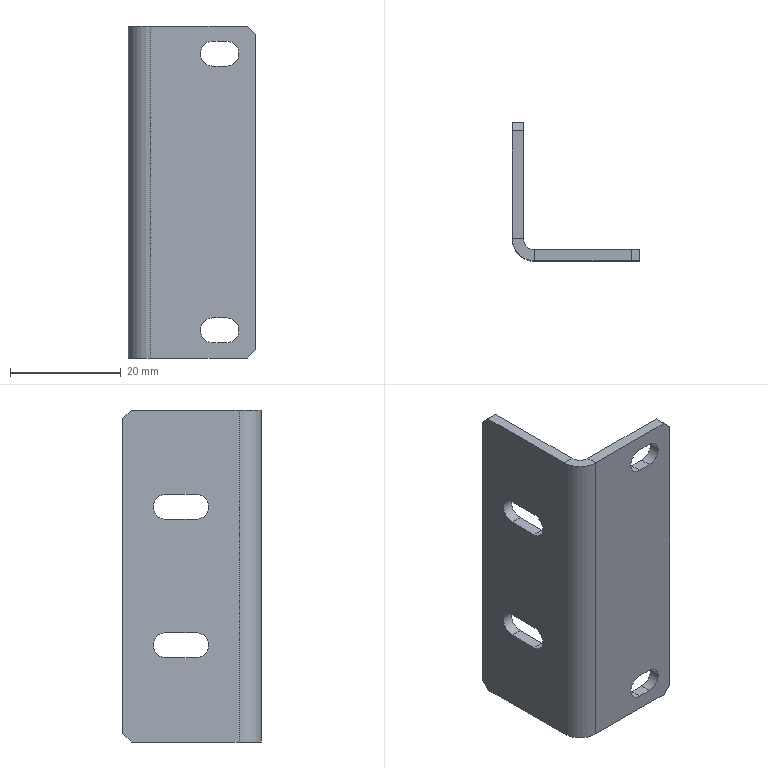Part | SolidWorks | features HoleWzd 2, Chamfer 1, FlatPattern 1, SMBaseFlange 1, SheetMetal 1 | 1 solid | 34 faces | box 23 x 25 x 60 mm | volume 5085 mm3 | plane 24 | cylinder 10 | commonest cylinder face diameters 4.5 x8 4 x1 8 x1
STEP:
#1=CARTESIAN_POINT('',(0.,-21.,60.));
#2=VERTEX_POINT('',#1);
#3=CARTESIAN_POINT('',(2.,-21.,60.));
#4=VERTEX_POINT('',#3);
#5=CARTESIAN_POINT('',(0.,-21.,60.));
#6=DIRECTION('',(1.,0.,0.));
#7=VECTOR('',#6,1000.);
#8=LINE('',#5,#7);
#9=EDGE_CURVE('',#2,#4,#8,.T.);
#10=ORIENTED_EDGE('',*,*,#9,.F.);
#11=CARTESIAN_POINT('',(4.,-25.,60.));
#12=VERTEX_POINT('',#11);
#13=CARTESIAN_POINT('',(4.,-21.,60.));
#14=DIRECTION('',(0.,0.,1.));
#15=DIRECTION('',(-1.,0.,0.));
#16=AXIS2_PLACEMENT_3D('',#13,#14,#15);
#17=CIRCLE('',#16,4.);
#18=EDGE_CURVE('',#2,#12,#17,.T.);
#19=ORIENTED_EDGE('',*,*,#18,.T.);
#20=CARTESIAN_POINT('',(4.,-23.,60.));
#21=VERTEX_POINT('',#20);
#22=CARTESIAN_POINT('',(4.,-23.,60.));
#23=DIRECTION('',(0.,-1.,0.));
#24=VECTOR('',#23,1000.);
#25=LINE('',#22,#24);
#26=EDGE_CURVE('',#21,#12,#25,.T.);
#27=ORIENTED_EDGE('',*,*,#26,.F.);
#28=CARTESIAN_POINT('',(4.,-21.,60.));
#29=DIRECTION('',(0.,0.,1.));
#30=DIRECTION('',(1.,0.,0.));
#31=AXIS2_PLACEMENT_3D('',#28,#29,#30);
#32=CIRCLE('',#31,2.);
#33=EDGE_CURVE('',#4,#21,#32,.T.);
#34=ORIENTED_EDGE('',*,*,#33,.F.);
#35=EDGE_LOOP('',(#10,#19,#27,#34));
#36=FACE_OUTER_BOUND('',#35,.T.);
#37=CARTESIAN_POINT('',(0.,-21.,60.));
#38=DIRECTION('',(0.,0.,1.));
#39=DIRECTION('',(1.,0.,0.));
#40=AXIS2_PLACEMENT_3D('',#37,#38,#39);
#41=PLANE('',#40);
#42=ADVANCED_FACE('',(#36),#41,.T.);
#43=CARTESIAN_POINT('',(2.,-1.5,60.));
#44=VERTEX_POINT('',#43);
#45=CARTESIAN_POINT('',(2.,0.,60.));
#46=DIRECTION('',(0.,-1.,0.));
#47=VECTOR('',#46,1000.);
#48=LINE('',#45,#47);
#49=EDGE_CURVE('',#44,#4,#48,.T.);
#50=ORIENTED_EDGE('',*,*,#49,.F.);
#51=CARTESIAN_POINT('',(0.,-1.5,60.));
#52=VERTEX_POINT('',#51);
#53=CARTESIAN_POINT('',(4.,-1.5,60.));
#54=DIRECTION('',(-1.,0.,0.));
#55=VECTOR('',#54,1000.);
#56=LINE('',#53,#55);
#57=EDGE_CURVE('',#44,#52,#56,.T.);
#58=ORIENTED_EDGE('',*,*,#57,.T.);
#59=CARTESIAN_POINT('',(0.,0.,60.));
#60=DIRECTION('',(0.,-1.,0.));
#61=VECTOR('',#60,1000.);
#62=LINE('',#59,#61);
#63=EDGE_CURVE('',#52,#2,#62,.T.);
#64=ORIENTED_EDGE('',*,*,#63,.T.);
#65=ORIENTED_EDGE('',*,*,#9,.T.);
#66=EDGE_LOOP('',(#50,#58,#64,#65));
#67=FACE_OUTER_BOUND('',#66,.T.);
#68=CARTESIAN_POINT('',(4.,-23.,60.));
#69=DIRECTION('',(0.,0.,1.));
#70=DIRECTION('',(1.,0.,0.));
#71=AXIS2_PLACEMENT_3D('',#68,#69,#70);
#72=PLANE('',#71);
#73=ADVANCED_FACE('',(#67),#72,.T.);
#74=CARTESIAN_POINT('',(4.,-25.,0.));
#75=VERTEX_POINT('',#74);
#76=CARTESIAN_POINT('',(4.,-23.,0.));
#77=VERTEX_POINT('',#76);
#78=CARTESIAN_POINT('',(4.,-25.,0.));
#79=DIRECTION('',(0.,1.,0.));
#80=VECTOR('',#79,1000.);
#81=LINE('',#78,#80);
#82=EDGE_CURVE('',#75,#77,#81,.T.);
#83=ORIENTED_EDGE('',*,*,#82,.F.);
#84=CARTESIAN_POINT('',(0.,-21.,0.));
#85=VERTEX_POINT('',#84);
#86=CARTESIAN_POINT('',(4.,-21.,0.));
#87=DIRECTION('',(0.,0.,1.));
#88=DIRECTION('',(-1.,0.,0.));
#89=AXIS2_PLACEMENT_3D('',#86,#87,#88);
#90=CIRCLE('',#89,4.);
#91=EDGE_CURVE('',#85,#75,#90,.T.);
#92=ORIENTED_EDGE('',*,*,#91,.F.);
#93=CARTESIAN_POINT('',(2.,-21.,0.));
#94=VERTEX_POINT('',#93);
#95=CARTESIAN_POINT('',(2.,-21.,0.));
#96=DIRECTION('',(-1.,0.,0.));
#97=VECTOR('',#96,1000.);
#98=LINE('',#95,#97);
#99=EDGE_CURVE('',#94,#85,#98,.T.);
#100=ORIENTED_EDGE('',*,*,#99,.F.);
#101=CARTESIAN_POINT('',(4.,-21.,0.));
#102=DIRECTION('',(0.,0.,1.));
#103=DIRECTION('',(1.,0.,0.));
#104=AXIS2_PLACEMENT_3D('',#101,#102,#103);
#105=CIRCLE('',#104,2.);
#106=EDGE_CURVE('',#94,#77,#105,.T.);
#107=ORIENTED_EDGE('',*,*,#106,.T.);
#108=EDGE_LOOP('',(#83,#92,#100,#107));
#109=FACE_OUTER_BOUND('',#108,.T.);
#110=CARTESIAN_POINT('',(4.,-25.,0.));
#111=DIRECTION('',(0.,0.,-1.));
#112=DIRECTION('',(-1.,0.,0.));
#113=AXIS2_PLACEMENT_3D('',#110,#111,#112);
#114=PLANE('',#113);
#115=ADVANCED_FACE('',(#109),#114,.T.);
#116=CARTESIAN_POINT('',(21.5,-23.,0.));
#117=VERTEX_POINT('',#116);
#118=CARTESIAN_POINT('',(0.,-23.,0.));
#119=DIRECTION('',(1.,0.,0.));
#120=VECTOR('',#119,1000.);
#121=LINE('',#118,#120);
#122=EDGE_CURVE('',#77,#117,#121,.T.);
#123=ORIENTED_EDGE('',*,*,#122,.T.);
#124=CARTESIAN_POINT('',(21.5,-25.,0.));
#125=VERTEX_POINT('',#124);
#126=CARTESIAN_POINT('',(21.5,-21.,0.));
#127=DIRECTION('',(0.,-1.,0.));
#128=VECTOR('',#127,1000.);
#129=LINE('',#126,#128);
#130=EDGE_CURVE('',#117,#125,#129,.T.);
#131=ORIENTED_EDGE('',*,*,#130,.T.);
#132=CARTESIAN_POINT('',(0.,-25.,0.));
#133=DIRECTION('',(1.,0.,0.));
#134=VECTOR('',#133,1000.);
#135=LINE('',#132,#134);
#136=EDGE_CURVE('',#75,#125,#135,.T.);
#137=ORIENTED_EDGE('',*,*,#136,.F.);
#138=ORIENTED_EDGE('',*,*,#82,.T.);
#139=EDGE_LOOP('',(#123,#131,#137,#138));
#140=FACE_OUTER_BOUND('',#139,.T.);
#141=CARTESIAN_POINT('',(2.,-21.,0.));
#142=DIRECTION('',(0.,0.,-1.));
#143=DIRECTION('',(-1.,0.,0.));
#144=AXIS2_PLACEMENT_3D('',#141,#142,#143);
#145=PLANE('',#144);
#146=ADVANCED_FACE('',(#140),#145,.T.);
#147=CARTESIAN_POINT('',(15.25,-25.,2.75));
#148=VERTEX_POINT('',#147);
#149=CARTESIAN_POINT('',(15.25,-25.,7.25));
#150=VERTEX_POINT('',#149);
#151=CARTESIAN_POINT('',(15.25,-25.,5.));
#152=DIRECTION('',(0.,1.,0.));
#153=DIRECTION('',(0.,0.,1.));
#154=AXIS2_PLACEMENT_3D('',#151,#152,#153);
#155=CIRCLE('',#154,2.25);
#156=EDGE_CURVE('',#148,#150,#155,.T.);
#157=ORIENTED_EDGE('',*,*,#156,.T.);
#158=CARTESIAN_POINT('',(17.75,-25.,7.25));
#159=VERTEX_POINT('',#158);
#160=CARTESIAN_POINT('',(0.,-25.,7.25));
#161=DIRECTION('',(1.,0.,0.));
#162=VECTOR('',#161,1000.);
#163=LINE('',#160,#162);
#164=EDGE_CURVE('',#150,#159,#163,.T.);
#165=ORIENTED_EDGE('',*,*,#164,.T.);
#166=CARTESIAN_POINT('',(17.75,-25.,2.75));
#167=VERTEX_POINT('',#166);
#168=CARTESIAN_POINT('',(17.75,-25.,5.));
#169=DIRECTION('',(0.,1.,0.));
#170=DIRECTION('',(0.,0.,1.));
#171=AXIS2_PLACEMENT_3D('',#168,#169,#170);
#172=CIRCLE('',#171,2.25);
#173=EDGE_CURVE('',#159,#167,#172,.T.);
#174=ORIENTED_EDGE('',*,*,#173,.T.);
#175=CARTESIAN_POINT('',(0.,-25.,2.75));
#176=DIRECTION('',(-1.,0.,0.));
#177=VECTOR('',#176,1000.);
#178=LINE('',#175,#177);
#179=EDGE_CURVE('',#167,#148,#178,.T.);
#180=ORIENTED_EDGE('',*,*,#179,.T.);
#181=EDGE_LOOP('',(#157,#165,#174,#180));
#182=FACE_BOUND('',#181,.T.);
#183=CARTESIAN_POINT('',(17.75,-25.,52.75));
#184=VERTEX_POINT('',#183);
#185=CARTESIAN_POINT('',(15.25,-25.,52.75));
#186=VERTEX_POINT('',#185);
#187=CARTESIAN_POINT('',(0.,-25.,52.75));
#188=DIRECTION('',(-1.,0.,0.));
#189=VECTOR('',#188,1000.);
#190=LINE('',#187,#189);
#191=EDGE_CURVE('',#184,#186,#190,.T.);
#192=ORIENTED_EDGE('',*,*,#191,.T.);
#193=CARTESIAN_POINT('',(15.25,-25.,57.25));
#194=VERTEX_POINT('',#193);
#195=CARTESIAN_POINT('',(15.25,-25.,55.));
#196=DIRECTION('',(0.,1.,0.));
#197=DIRECTION('',(0.,0.,1.));
#198=AXIS2_PLACEMENT_3D('',#195,#196,#197);
#199=CIRCLE('',#198,2.25);
#200=EDGE_CURVE('',#186,#194,#199,.T.);
#201=ORIENTED_EDGE('',*,*,#200,.T.);
#202=CARTESIAN_POINT('',(17.75,-25.,57.25));
#203=VERTEX_POINT('',#202);
#204=CARTESIAN_POINT('',(0.,-25.,57.25));
#205=DIRECTION('',(1.,0.,0.));
#206=VECTOR('',#205,1000.);
#207=LINE('',#204,#206);
#208=EDGE_CURVE('',#194,#203,#207,.T.);
#209=ORIENTED_EDGE('',*,*,#208,.T.);
#210=CARTESIAN_POINT('',(17.75,-25.,55.));
#211=DIRECTION('',(0.,1.,0.));
#212=DIRECTION('',(0.,0.,1.));
#213=AXIS2_PLACEMENT_3D('',#210,#211,#212);
#214=CIRCLE('',#213,2.25);
#215=EDGE_CURVE('',#203,#184,#214,.T.);
#216=ORIENTED_EDGE('',*,*,#215,.T.);
#217=EDGE_LOOP('',(#192,#201,#209,#216));
#218=FACE_BOUND('',#217,.T.);
#219=CARTESIAN_POINT('',(23.,-25.,58.5));
#220=VERTEX_POINT('',#219);
#221=CARTESIAN_POINT('',(23.,-25.,1.5));
#222=VERTEX_POINT('',#221);
#223=CARTESIAN_POINT('',(23.,-25.,60.));
#224=DIRECTION('',(0.,0.,-1.));
#225=VECTOR('',#224,1000.);
#226=LINE('',#223,#225);
#227=EDGE_CURVE('',#220,#222,#226,.T.);
#228=ORIENTED_EDGE('',*,*,#227,.F.);
#229=CARTESIAN_POINT('',(21.5,-25.,60.));
#230=VERTEX_POINT('',#229);
#231=CARTESIAN_POINT('',(23.,-25.,58.5));
#232=DIRECTION('',(-0.7071,0.,0.7071));
#233=VECTOR('',#232,1000.);
#234=LINE('',#231,#233);
#235=EDGE_CURVE('',#220,#230,#234,.T.);
#236=ORIENTED_EDGE('',*,*,#235,.T.);
#237=CARTESIAN_POINT('',(0.,-25.,60.));
#238=DIRECTION('',(1.,0.,0.));
#239=VECTOR('',#238,1000.);
#240=LINE('',#237,#239);
#241=EDGE_CURVE('',#12,#230,#240,.T.);
#242=ORIENTED_EDGE('',*,*,#241,.F.);
#243=CARTESIAN_POINT('',(4.,-25.,60.));
#244=DIRECTION('',(0.,0.,-1.));
#245=VECTOR('',#244,1000.);
#246=LINE('',#243,#245);
#247=EDGE_CURVE('',#12,#75,#246,.T.);
#248=ORIENTED_EDGE('',*,*,#247,.T.);
#249=ORIENTED_EDGE('',*,*,#136,.T.);
#250=CARTESIAN_POINT('',(21.5,-25.,0.));
#251=DIRECTION('',(0.7071,0.,0.7071));
#252=VECTOR('',#251,1000.);
#253=LINE('',#250,#252);
#254=EDGE_CURVE('',#125,#222,#253,.T.);
#255=ORIENTED_EDGE('',*,*,#254,.T.);
#256=EDGE_LOOP('',(#228,#236,#242,#248,#249,#255));
#257=FACE_OUTER_BOUND('',#256,.T.);
#258=CARTESIAN_POINT('',(0.,-25.,60.));
#259=DIRECTION('',(0.,1.,0.));
#260=DIRECTION('',(0.,0.,1.));
#261=AXIS2_PLACEMENT_3D('',#258,#259,#260);
#262=PLANE('',#261);
#263=ADVANCED_FACE('',(#182,#218,#257),#262,.F.);
#264=CARTESIAN_POINT('',(23.,-23.,58.5));
#265=VERTEX_POINT('',#264);
#266=CARTESIAN_POINT('',(23.,-23.,1.5));
#267=VERTEX_POINT('',#266);
#268=CARTESIAN_POINT('',(23.,-23.,60.));
#269=DIRECTION('',(0.,0.,-1.));
#270=VECTOR('',#269,1000.);
#271=LINE('',#268,#270);
#272=EDGE_CURVE('',#265,#267,#271,.T.);
#273=ORIENTED_EDGE('',*,*,#272,.F.);
#274=CARTESIAN_POINT('',(23.,-23.,58.5));
#275=DIRECTION('',(0.,-1.,0.));
#276=VECTOR('',#275,1000.);
#277=LINE('',#274,#276);
#278=EDGE_CURVE('',#265,#220,#277,.T.);
#279=ORIENTED_EDGE('',*,*,#278,.T.);
#280=ORIENTED_EDGE('',*,*,#227,.T.);
#281=CARTESIAN_POINT('',(23.,-23.,1.5));
#282=DIRECTION('',(0.,1.,0.));
#283=VECTOR('',#282,1000.);
#284=LINE('',#281,#283);
#285=EDGE_CURVE('',#222,#267,#284,.T.);
#286=ORIENTED_EDGE('',*,*,#285,.T.);
#287=EDGE_LOOP('',(#273,#279,#280,#286));
#288=FACE_OUTER_BOUND('',#287,.T.);
#289=CARTESIAN_POINT('',(23.,-23.,60.));
#290=DIRECTION('',(1.,0.,0.));
#291=DIRECTION('',(0.,0.,-1.));
#292=AXIS2_PLACEMENT_3D('',#289,#290,#291);
#293=PLANE('',#292);
#294=ADVANCED_FACE('',(#288),#293,.T.);
#295=CARTESIAN_POINT('',(15.25,-23.,7.25));
#296=VERTEX_POINT('',#295);
#297=CARTESIAN_POINT('',(17.75,-23.,7.25));
#298=VERTEX_POINT('',#297);
#299=CARTESIAN_POINT('',(15.25,-23.,7.25));
#300=DIRECTION('',(1.,0.,0.));
#301=VECTOR('',#300,1000.);
#302=LINE('',#299,#301);
#303=EDGE_CURVE('',#296,#298,#302,.T.);
#304=ORIENTED_EDGE('',*,*,#303,.F.);
#305=CARTESIAN_POINT('',(15.25,-23.,2.75));
#306=VERTEX_POINT('',#305);
#307=CARTESIAN_POINT('',(15.25,-23.,5.));
#308=DIRECTION('',(0.,1.,0.));
#309=DIRECTION('',(0.,0.,1.));
#310=AXIS2_PLACEMENT_3D('',#307,#308,#309);
#311=CIRCLE('',#310,2.25);
#312=EDGE_CURVE('',#306,#296,#311,.T.);
#313=ORIENTED_EDGE('',*,*,#312,.F.);
#314=CARTESIAN_POINT('',(17.75,-23.,2.75));
#315=VERTEX_POINT('',#314);
#316=CARTESIAN_POINT('',(15.25,-23.,2.75));
#317=DIRECTION('',(1.,0.,0.));
#318=VECTOR('',#317,1000.);
#319=LINE('',#316,#318);
#320=EDGE_CURVE('',#306,#315,#319,.T.);
#321=ORIENTED_EDGE('',*,*,#320,.T.);
#322=CARTESIAN_POINT('',(17.75,-23.,5.));
#323=DIRECTION('',(0.,1.,0.));
#324=DIRECTION('',(0.,0.,1.));
#325=AXIS2_PLACEMENT_3D('',#322,#323,#324);
#326=CIRCLE('',#325,2.25);
#327=EDGE_CURVE('',#298,#315,#326,.T.);
#328=ORIENTED_EDGE('',*,*,#327,.F.);
#329=EDGE_LOOP('',(#304,#313,#321,#328));
#330=FACE_BOUND('',#329,.T.);
#331=CARTESIAN_POINT('',(17.75,-23.,57.25));
#332=VERTEX_POINT('',#331);
#333=CARTESIAN_POINT('',(17.75,-23.,52.75));
#334=VERTEX_POINT('',#333);
#335=CARTESIAN_POINT('',(17.75,-23.,55.));
#336=DIRECTION('',(0.,1.,0.));
#337=DIRECTION('',(0.,0.,1.));
#338=AXIS2_PLACEMENT_3D('',#335,#336,#337);
#339=CIRCLE('',#338,2.25);
#340=EDGE_CURVE('',#332,#334,#339,.T.);
#341=ORIENTED_EDGE('',*,*,#340,.F.);
#342=CARTESIAN_POINT('',(15.25,-23.,57.25));
#343=VERTEX_POINT('',#342);
#344=CARTESIAN_POINT('',(15.25,-23.,57.25));
#345=DIRECTION('',(1.,0.,0.));
#346=VECTOR('',#345,1000.);
#347=LINE('',#344,#346);
#348=EDGE_CURVE('',#343,#332,#347,.T.);
#349=ORIENTED_EDGE('',*,*,#348,.F.);
#350=CARTESIAN_POINT('',(15.25,-23.,52.75));
#351=VERTEX_POINT('',#350);
#352=CARTESIAN_POINT('',(15.25,-23.,55.));
#353=DIRECTION('',(0.,1.,0.));
#354=DIRECTION('',(0.,0.,1.));
#355=AXIS2_PLACEMENT_3D('',#352,#353,#354);
#356=CIRCLE('',#355,2.25);
#357=EDGE_CURVE('',#351,#343,#356,.T.);
#358=ORIENTED_EDGE('',*,*,#357,.F.);
#359=CARTESIAN_POINT('',(15.25,-23.,52.75));
#360=DIRECTION('',(1.,0.,0.));
#361=VECTOR('',#360,1000.);
#362=LINE('',#359,#361);
#363=EDGE_CURVE('',#351,#334,#362,.T.);
#364=ORIENTED_EDGE('',*,*,#363,.T.);
#365=EDGE_LOOP('',(#341,#349,#358,#364));
#366=FACE_BOUND('',#365,.T.);
#367=CARTESIAN_POINT('',(21.5,-23.,60.));
#368=VERTEX_POINT('',#367);
#369=CARTESIAN_POINT('',(0.,-23.,60.));
#370=DIRECTION('',(1.,0.,0.));
#371=VECTOR('',#370,1000.);
#372=LINE('',#369,#371);
#373=EDGE_CURVE('',#21,#368,#372,.T.);
#374=ORIENTED_EDGE('',*,*,#373,.T.);
#375=CARTESIAN_POINT('',(10.75,-23.,70.75));
#376=DIRECTION('',(0.7071,0.,-0.7071));
#377=VECTOR('',#376,1000.);
#378=LINE('',#375,#377);
#379=EDGE_CURVE('',#368,#265,#378,.T.);
#380=ORIENTED_EDGE('',*,*,#379,.T.);
#381=ORIENTED_EDGE('',*,*,#272,.T.);
#382=CARTESIAN_POINT('',(40.75,-23.,19.25));
#383=DIRECTION('',(-0.7071,0.,-0.7071));
#384=VECTOR('',#383,1000.);
#385=LINE('',#382,#384);
#386=EDGE_CURVE('',#267,#117,#385,.T.);
#387=ORIENTED_EDGE('',*,*,#386,.T.);
#388=ORIENTED_EDGE('',*,*,#122,.F.);
#389=CARTESIAN_POINT('',(4.,-23.,60.));
#390=DIRECTION('',(0.,0.,-1.));
#391=VECTOR('',#390,1000.);
#392=LINE('',#389,#391);
#393=EDGE_CURVE('',#21,#77,#392,.T.);
#394=ORIENTED_EDGE('',*,*,#393,.F.);
#395=EDGE_LOOP('',(#374,#380,#381,#387,#388,#394));
#396=FACE_OUTER_BOUND('',#395,.T.);
#397=CARTESIAN_POINT('',(0.,-23.,60.));
#398=DIRECTION('',(0.,1.,0.));
#399=DIRECTION('',(0.,0.,1.));
#400=AXIS2_PLACEMENT_3D('',#397,#398,#399);
#401=PLANE('',#400);
#402=ADVANCED_FACE('',(#330,#366,#396),#401,.T.);
#403=ORIENTED_EDGE('',*,*,#106,.F.);
#404=CARTESIAN_POINT('',(2.,-21.,60.));
#405=DIRECTION('',(0.,0.,-1.));
#406=VECTOR('',#405,1000.);
#407=LINE('',#404,#406);
#408=EDGE_CURVE('',#4,#94,#407,.T.);
#409=ORIENTED_EDGE('',*,*,#408,.F.);
#410=ORIENTED_EDGE('',*,*,#33,.T.);
#411=ORIENTED_EDGE('',*,*,#393,.T.);
#412=EDGE_LOOP('',(#403,#409,#410,#411));
#413=FACE_OUTER_BOUND('',#412,.T.);
#414=CARTESIAN_POINT('',(4.,-21.,60.));
#415=DIRECTION('',(0.,0.,-1.));
#416=DIRECTION('',(-1.,0.,0.));
#417=AXIS2_PLACEMENT_3D('',#414,#415,#416);
#418=CYLINDRICAL_SURFACE('',#417,2.);
#419=ADVANCED_FACE('',(#413),#418,.F.);
#420=CARTESIAN_POINT('',(2.,-13.25,19.75));
#421=VERTEX_POINT('',#420);
#422=CARTESIAN_POINT('',(2.,-13.25,15.25));
#423=VERTEX_POINT('',#422);
#424=CARTESIAN_POINT('',(2.,-13.25,17.5));
#425=DIRECTION('',(1.,0.,0.));
#426=DIRECTION('',(0.,0.,-1.));
#427=AXIS2_PLACEMENT_3D('',#424,#425,#426);
#428=CIRCLE('',#427,2.25);
#429=EDGE_CURVE('',#421,#423,#428,.T.);
#430=ORIENTED_EDGE('',*,*,#429,.F.);
#431=CARTESIAN_POINT('',(2.,-7.75,19.75));
#432=VERTEX_POINT('',#431);
#433=CARTESIAN_POINT('',(2.,-13.25,19.75));
#434=DIRECTION('',(0.,1.,0.));
#435=VECTOR('',#434,1000.);
#436=LINE('',#433,#435);
#437=EDGE_CURVE('',#421,#432,#436,.T.);
#438=ORIENTED_EDGE('',*,*,#437,.T.);
#439=CARTESIAN_POINT('',(2.,-7.75,15.25));
#440=VERTEX_POINT('',#439);
#441=CARTESIAN_POINT('',(2.,-7.75,17.5));
#442=DIRECTION('',(1.,0.,0.));
#443=DIRECTION('',(0.,0.,-1.));
#444=AXIS2_PLACEMENT_3D('',#441,#442,#443);
#445=CIRCLE('',#444,2.25);
#446=EDGE_CURVE('',#440,#432,#445,.T.);
#447=ORIENTED_EDGE('',*,*,#446,.F.);
#448=CARTESIAN_POINT('',(2.,-13.25,15.25));
#449=DIRECTION('',(0.,1.,0.));
#450=VECTOR('',#449,1000.);
#451=LINE('',#448,#450);
#452=EDGE_CURVE('',#423,#440,#451,.T.);
#453=ORIENTED_EDGE('',*,*,#452,.F.);
#454=EDGE_LOOP('',(#430,#438,#447,#453));
#455=FACE_BOUND('',#454,.T.);
#456=CARTESIAN_POINT('',(2.,-7.75,40.25));
#457=VERTEX_POINT('',#456);
#458=CARTESIAN_POINT('',(2.,-7.75,44.75));
#459=VERTEX_POINT('',#458);
#460=CARTESIAN_POINT('',(2.,-7.75,42.5));
#461=DIRECTION('',(1.,0.,0.));
#462=DIRECTION('',(0.,0.,-1.));
#463=AXIS2_PLACEMENT_3D('',#460,#461,#462);
#464=CIRCLE('',#463,2.25);
#465=EDGE_CURVE('',#457,#459,#464,.T.);
#466=ORIENTED_EDGE('',*,*,#465,.F.);
#467=CARTESIAN_POINT('',(2.,-13.25,40.25));
#468=VERTEX_POINT('',#467);
#469=CARTESIAN_POINT('',(2.,-13.25,40.25));
#470=DIRECTION('',(0.,1.,0.));
#471=VECTOR('',#470,1000.);
#472=LINE('',#469,#471);
#473=EDGE_CURVE('',#468,#457,#472,.T.);
#474=ORIENTED_EDGE('',*,*,#473,.F.);
#475=CARTESIAN_POINT('',(2.,-13.25,44.75));
#476=VERTEX_POINT('',#475);
#477=CARTESIAN_POINT('',(2.,-13.25,42.5));
#478=DIRECTION('',(1.,0.,0.));
#479=DIRECTION('',(0.,0.,-1.));
#480=AXIS2_PLACEMENT_3D('',#477,#478,#479);
#481=CIRCLE('',#480,2.25);
#482=EDGE_CURVE('',#476,#468,#481,.T.);
#483=ORIENTED_EDGE('',*,*,#482,.F.);
#484=CARTESIAN_POINT('',(2.,-13.25,44.75));
#485=DIRECTION('',(0.,1.,0.));
#486=VECTOR('',#485,1000.);
#487=LINE('',#484,#486);
#488=EDGE_CURVE('',#476,#459,#487,.T.);
#489=ORIENTED_EDGE('',*,*,#488,.T.);
#490=EDGE_LOOP('',(#466,#474,#483,#489));
#491=FACE_BOUND('',#490,.T.);
#492=CARTESIAN_POINT('',(2.,0.,58.5));
#493=VERTEX_POINT('',#492);
#494=CARTESIAN_POINT('',(2.,0.,1.5));
#495=VERTEX_POINT('',#494);
#496=CARTESIAN_POINT('',(2.,0.,60.));
#497=DIRECTION('',(0.,0.,-1.));
#498=VECTOR('',#497,1000.);
#499=LINE('',#496,#498);
#500=EDGE_CURVE('',#493,#495,#499,.T.);
#501=ORIENTED_EDGE('',*,*,#500,.F.);
#502=CARTESIAN_POINT('',(2.,-0.75,59.25));
#503=DIRECTION('',(0.,-0.7071,0.7071));
#504=VECTOR('',#503,1000.);
#505=LINE('',#502,#504);
#506=EDGE_CURVE('',#493,#44,#505,.T.);
#507=ORIENTED_EDGE('',*,*,#506,.T.);
#508=ORIENTED_EDGE('',*,*,#49,.T.);
#509=ORIENTED_EDGE('',*,*,#408,.T.);
#510=CARTESIAN_POINT('',(2.,-1.5,0.));
#511=VERTEX_POINT('',#510);
#512=CARTESIAN_POINT('',(2.,0.,0.));
#513=DIRECTION('',(0.,-1.,0.));
#514=VECTOR('',#513,1000.);
#515=LINE('',#512,#514);
#516=EDGE_CURVE('',#511,#94,#515,.T.);
#517=ORIENTED_EDGE('',*,*,#516,.F.);
#518=CARTESIAN_POINT('',(2.,29.25,30.75));
#519=DIRECTION('',(0.,0.7071,0.7071));
#520=VECTOR('',#519,1000.);
#521=LINE('',#518,#520);
#522=EDGE_CURVE('',#511,#495,#521,.T.);
#523=ORIENTED_EDGE('',*,*,#522,.T.);
#524=EDGE_LOOP('',(#501,#507,#508,#509,#517,#523));
#525=FACE_OUTER_BOUND('',#524,.T.);
#526=CARTESIAN_POINT('',(2.,0.,60.));
#527=DIRECTION('',(1.,0.,0.));
#528=DIRECTION('',(0.,1.,0.));
#529=AXIS2_PLACEMENT_3D('',#526,#527,#528);
#530=PLANE('',#529);
#531=ADVANCED_FACE('',(#455,#491,#525),#530,.T.);
#532=CARTESIAN_POINT('',(0.,0.,58.5));
#533=VERTEX_POINT('',#532);
#534=CARTESIAN_POINT('',(0.,0.,1.5));
#535=VERTEX_POINT('',#534);
#536=CARTESIAN_POINT('',(0.,0.,60.));
#537=DIRECTION('',(0.,0.,-1.));
#538=VECTOR('',#537,1000.);
#539=LINE('',#536,#538);
#540=EDGE_CURVE('',#533,#535,#539,.T.);
#541=ORIENTED_EDGE('',*,*,#540,.F.);
#542=CARTESIAN_POINT('',(0.,0.,58.5));
#543=DIRECTION('',(1.,0.,0.));
#544=VECTOR('',#543,1000.);
#545=LINE('',#542,#544);
#546=EDGE_CURVE('',#533,#493,#545,.T.);
#547=ORIENTED_EDGE('',*,*,#546,.T.);
#548=ORIENTED_EDGE('',*,*,#500,.T.);
#549=CARTESIAN_POINT('',(0.,0.,1.5));
#550=DIRECTION('',(-1.,0.,0.));
#551=VECTOR('',#550,1000.);
#552=LINE('',#549,#551);
#553=EDGE_CURVE('',#495,#535,#552,.T.);
#554=ORIENTED_EDGE('',*,*,#553,.T.);
#555=EDGE_LOOP('',(#541,#547,#548,#554));
#556=FACE_OUTER_BOUND('',#555,.T.);
#557=CARTESIAN_POINT('',(0.,0.,60.));
#558=DIRECTION('',(0.,1.,0.));
#559=DIRECTION('',(-1.,0.,0.));
#560=AXIS2_PLACEMENT_3D('',#557,#558,#559);
#561=PLANE('',#560);
#562=ADVANCED_FACE('',(#556),#561,.T.);
#563=CARTESIAN_POINT('',(0.,-13.25,15.25));
#564=VERTEX_POINT('',#563);
#565=CARTESIAN_POINT('',(0.,-7.75,15.25));
#566=VERTEX_POINT('',#565);
#567=CARTESIAN_POINT('',(0.,0.,15.25));
#568=DIRECTION('',(0.,1.,0.));
#569=VECTOR('',#568,1000.);
#570=LINE('',#567,#569);
#571=EDGE_CURVE('',#564,#566,#570,.T.);
#572=ORIENTED_EDGE('',*,*,#571,.T.);
#573=CARTESIAN_POINT('',(0.,-7.75,19.75));
#574=VERTEX_POINT('',#573);
#575=CARTESIAN_POINT('',(0.,-7.75,17.5));
#576=DIRECTION('',(1.,0.,0.));
#577=DIRECTION('',(0.,1.,0.));
#578=AXIS2_PLACEMENT_3D('',#575,#576,#577);
#579=CIRCLE('',#578,2.25);
#580=EDGE_CURVE('',#566,#574,#579,.T.);
#581=ORIENTED_EDGE('',*,*,#580,.T.);
#582=CARTESIAN_POINT('',(0.,-13.25,19.75));
#583=VERTEX_POINT('',#582);
#584=CARTESIAN_POINT('',(0.,0.,19.75));
#585=DIRECTION('',(0.,-1.,0.));
#586=VECTOR('',#585,1000.);
#587=LINE('',#584,#586);
#588=EDGE_CURVE('',#574,#583,#587,.T.);
#589=ORIENTED_EDGE('',*,*,#588,.T.);
#590=CARTESIAN_POINT('',(0.,-13.25,17.5));
#591=DIRECTION('',(1.,0.,0.));
#592=DIRECTION('',(0.,1.,0.));
#593=AXIS2_PLACEMENT_3D('',#590,#591,#592);
#594=CIRCLE('',#593,2.25);
#595=EDGE_CURVE('',#583,#564,#594,.T.);
#596=ORIENTED_EDGE('',*,*,#595,.T.);
#597=EDGE_LOOP('',(#572,#581,#589,#596));
#598=FACE_BOUND('',#597,.T.);
#599=CARTESIAN_POINT('',(0.,-13.25,44.75));
#600=VERTEX_POINT('',#599);
#601=CARTESIAN_POINT('',(0.,-13.25,40.25));
#602=VERTEX_POINT('',#601);
#603=CARTESIAN_POINT('',(0.,-13.25,42.5));
#604=DIRECTION('',(1.,0.,0.));
#605=DIRECTION('',(0.,1.,0.));
#606=AXIS2_PLACEMENT_3D('',#603,#604,#605);
#607=CIRCLE('',#606,2.25);
#608=EDGE_CURVE('',#600,#602,#607,.T.);
#609=ORIENTED_EDGE('',*,*,#608,.T.);
#610=CARTESIAN_POINT('',(0.,-7.75,40.25));
#611=VERTEX_POINT('',#610);
#612=CARTESIAN_POINT('',(0.,0.,40.25));
#613=DIRECTION('',(0.,1.,0.));
#614=VECTOR('',#613,1000.);
#615=LINE('',#612,#614);
#616=EDGE_CURVE('',#602,#611,#615,.T.);
#617=ORIENTED_EDGE('',*,*,#616,.T.);
#618=CARTESIAN_POINT('',(0.,-7.75,44.75));
#619=VERTEX_POINT('',#618);
#620=CARTESIAN_POINT('',(0.,-7.75,42.5));
#621=DIRECTION('',(1.,0.,0.));
#622=DIRECTION('',(0.,1.,0.));
#623=AXIS2_PLACEMENT_3D('',#620,#621,#622);
#624=CIRCLE('',#623,2.25);
#625=EDGE_CURVE('',#611,#619,#624,.T.);
#626=ORIENTED_EDGE('',*,*,#625,.T.);
#627=CARTESIAN_POINT('',(0.,0.,44.75));
#628=DIRECTION('',(0.,-1.,0.));
#629=VECTOR('',#628,1000.);
#630=LINE('',#627,#629);
#631=EDGE_CURVE('',#619,#600,#630,.T.);
#632=ORIENTED_EDGE('',*,*,#631,.T.);
#633=EDGE_LOOP('',(#609,#617,#626,#632));
#634=FACE_BOUND('',#633,.T.);
#635=ORIENTED_EDGE('',*,*,#63,.F.);
#636=CARTESIAN_POINT('',(0.,0.,58.5));
#637=DIRECTION('',(0.,0.7071,-0.7071));
#638=VECTOR('',#637,1000.);
#639=LINE('',#636,#638);
#640=EDGE_CURVE('',#52,#533,#639,.T.);
#641=ORIENTED_EDGE('',*,*,#640,.T.);
#642=ORIENTED_EDGE('',*,*,#540,.T.);
#643=CARTESIAN_POINT('',(0.,-1.5,0.));
#644=VERTEX_POINT('',#643);
#645=CARTESIAN_POINT('',(0.,-1.5,0.));
#646=DIRECTION('',(0.,-0.7071,-0.7071));
#647=VECTOR('',#646,1000.);
#648=LINE('',#645,#647);
#649=EDGE_CURVE('',#535,#644,#648,.T.);
#650=ORIENTED_EDGE('',*,*,#649,.T.);
#651=CARTESIAN_POINT('',(0.,0.,0.));
#652=DIRECTION('',(0.,-1.,0.));
#653=VECTOR('',#652,1000.);
#654=LINE('',#651,#653);
#655=EDGE_CURVE('',#644,#85,#654,.T.);
#656=ORIENTED_EDGE('',*,*,#655,.T.);
#657=CARTESIAN_POINT('',(0.,-21.,60.));
#658=DIRECTION('',(0.,0.,-1.));
#659=VECTOR('',#658,1000.);
#660=LINE('',#657,#659);
#661=EDGE_CURVE('',#2,#85,#660,.T.);
#662=ORIENTED_EDGE('',*,*,#661,.F.);
#663=EDGE_LOOP('',(#635,#641,#642,#650,#656,#662));
#664=FACE_OUTER_BOUND('',#663,.T.);
#665=CARTESIAN_POINT('',(0.,0.,60.));
#666=DIRECTION('',(1.,0.,0.));
#667=DIRECTION('',(0.,1.,0.));
#668=AXIS2_PLACEMENT_3D('',#665,#666,#667);
#669=PLANE('',#668);
#670=ADVANCED_FACE('',(#598,#634,#664),#669,.F.);
#671=ORIENTED_EDGE('',*,*,#91,.T.);
#672=ORIENTED_EDGE('',*,*,#247,.F.);
#673=ORIENTED_EDGE('',*,*,#18,.F.);
#674=ORIENTED_EDGE('',*,*,#661,.T.);
#675=EDGE_LOOP('',(#671,#672,#673,#674));
#676=FACE_OUTER_BOUND('',#675,.T.);
#677=CARTESIAN_POINT('',(4.,-21.,60.));
#678=DIRECTION('',(0.,0.,-1.));
#679=DIRECTION('',(-1.,0.,0.));
#680=AXIS2_PLACEMENT_3D('',#677,#678,#679);
#681=CYLINDRICAL_SURFACE('',#680,4.);
#682=ADVANCED_FACE('',(#676),#681,.T.);
#683=ORIENTED_EDGE('',*,*,#241,.T.);
#684=CARTESIAN_POINT('',(21.5,-21.,60.));
#685=DIRECTION('',(0.,1.,0.));
#686=VECTOR('',#685,1000.);
#687=LINE('',#684,#686);
#688=EDGE_CURVE('',#230,#368,#687,.T.);
#689=ORIENTED_EDGE('',*,*,#688,.T.);
#690=ORIENTED_EDGE('',*,*,#373,.F.);
#691=ORIENTED_EDGE('',*,*,#26,.T.);
#692=EDGE_LOOP('',(#683,#689,#690,#691));
#693=FACE_OUTER_BOUND('',#692,.T.);
#694=CARTESIAN_POINT('',(4.,-21.,60.));
#695=DIRECTION('',(0.,0.,1.));
#696=DIRECTION('',(1.,0.,0.));
#697=AXIS2_PLACEMENT_3D('',#694,#695,#696);
#698=PLANE('',#697);
#699=ADVANCED_FACE('',(#693),#698,.T.);
#700=ORIENTED_EDGE('',*,*,#655,.F.);
#701=CARTESIAN_POINT('',(2.,-1.5,0.));
#702=DIRECTION('',(1.,0.,0.));
#703=VECTOR('',#702,1000.);
#704=LINE('',#701,#703);
#705=EDGE_CURVE('',#644,#511,#704,.T.);
#706=ORIENTED_EDGE('',*,*,#705,.T.);
#707=ORIENTED_EDGE('',*,*,#516,.T.);
#708=ORIENTED_EDGE('',*,*,#99,.T.);
#709=EDGE_LOOP('',(#700,#706,#707,#708));
#710=FACE_OUTER_BOUND('',#709,.T.);
#711=CARTESIAN_POINT('',(4.,-21.,0.));
#712=DIRECTION('',(0.,0.,1.));
#713=DIRECTION('',(1.,0.,0.));
#714=AXIS2_PLACEMENT_3D('',#711,#712,#713);
#715=PLANE('',#714);
#716=ADVANCED_FACE('',(#710),#715,.F.);
#717=CARTESIAN_POINT('',(15.25,-23.,52.75));
#718=DIRECTION('',(0.,-1.,0.));
#719=VECTOR('',#718,1000.);
#720=LINE('',#717,#719);
#721=EDGE_CURVE('',#351,#186,#720,.T.);
#722=ORIENTED_EDGE('',*,*,#721,.F.);
#723=ORIENTED_EDGE('',*,*,#357,.T.);
#724=CARTESIAN_POINT('',(15.25,-23.,57.25));
#725=DIRECTION('',(0.,1.,0.));
#726=VECTOR('',#725,1000.);
#727=LINE('',#724,#726);
#728=EDGE_CURVE('',#194,#343,#727,.T.);
#729=ORIENTED_EDGE('',*,*,#728,.F.);
#730=ORIENTED_EDGE('',*,*,#200,.F.);
#731=EDGE_LOOP('',(#722,#723,#729,#730));
#732=FACE_OUTER_BOUND('',#731,.T.);
#733=CARTESIAN_POINT('',(15.25,-23.,55.));
#734=DIRECTION('',(0.,1.,0.));
#735=DIRECTION('',(0.,0.,1.));
#736=AXIS2_PLACEMENT_3D('',#733,#734,#735);
#737=CYLINDRICAL_SURFACE('',#736,2.25);
#738=ADVANCED_FACE('',(#732),#737,.F.);
#739=CARTESIAN_POINT('',(17.75,-23.,57.25));
#740=DIRECTION('',(0.,-1.,0.));
#741=VECTOR('',#740,1000.);
#742=LINE('',#739,#741);
#743=EDGE_CURVE('',#332,#203,#742,.T.);
#744=ORIENTED_EDGE('',*,*,#743,.F.);
#745=ORIENTED_EDGE('',*,*,#340,.T.);
#746=CARTESIAN_POINT('',(17.75,-23.,52.75));
#747=DIRECTION('',(0.,1.,0.));
#748=VECTOR('',#747,1000.);
#749=LINE('',#746,#748);
#750=EDGE_CURVE('',#184,#334,#749,.T.);
#751=ORIENTED_EDGE('',*,*,#750,.F.);
#752=ORIENTED_EDGE('',*,*,#215,.F.);
#753=EDGE_LOOP('',(#744,#745,#751,#752));
#754=FACE_OUTER_BOUND('',#753,.T.);
#755=CARTESIAN_POINT('',(17.75,-23.,55.));
#756=DIRECTION('',(0.,1.,0.));
#757=DIRECTION('',(0.,0.,1.));
#758=AXIS2_PLACEMENT_3D('',#755,#756,#757);
#759=CYLINDRICAL_SURFACE('',#758,2.25);
#760=ADVANCED_FACE('',(#754),#759,.F.);
#761=ORIENTED_EDGE('',*,*,#728,.T.);
#762=ORIENTED_EDGE('',*,*,#348,.T.);
#763=ORIENTED_EDGE('',*,*,#743,.T.);
#764=ORIENTED_EDGE('',*,*,#208,.F.);
#765=EDGE_LOOP('',(#761,#762,#763,#764));
#766=FACE_OUTER_BOUND('',#765,.T.);
#767=CARTESIAN_POINT('',(15.25,-23.,57.25));
#768=DIRECTION('',(0.,0.,1.));
#769=DIRECTION('',(1.,0.,0.));
#770=AXIS2_PLACEMENT_3D('',#767,#768,#769);
#771=PLANE('',#770);
#772=ADVANCED_FACE('',(#766),#771,.F.);
#773=ORIENTED_EDGE('',*,*,#750,.T.);
#774=ORIENTED_EDGE('',*,*,#363,.F.);
#775=ORIENTED_EDGE('',*,*,#721,.T.);
#776=ORIENTED_EDGE('',*,*,#191,.F.);
#777=EDGE_LOOP('',(#773,#774,#775,#776));
#778=FACE_OUTER_BOUND('',#777,.T.);
#779=CARTESIAN_POINT('',(15.25,-23.,52.75));
#780=DIRECTION('',(0.,0.,-1.));
#781=DIRECTION('',(-1.,0.,0.));
#782=AXIS2_PLACEMENT_3D('',#779,#780,#781);
#783=PLANE('',#782);
#784=ADVANCED_FACE('',(#778),#783,.F.);
#785=CARTESIAN_POINT('',(15.25,-23.,2.75));
#786=DIRECTION('',(0.,-1.,0.));
#787=VECTOR('',#786,1000.);
#788=LINE('',#785,#787);
#789=EDGE_CURVE('',#306,#148,#788,.T.);
#790=ORIENTED_EDGE('',*,*,#789,.F.);
#791=ORIENTED_EDGE('',*,*,#312,.T.);
#792=CARTESIAN_POINT('',(15.25,-23.,7.25));
#793=DIRECTION('',(0.,1.,0.));
#794=VECTOR('',#793,1000.);
#795=LINE('',#792,#794);
#796=EDGE_CURVE('',#150,#296,#795,.T.);
#797=ORIENTED_EDGE('',*,*,#796,.F.);
#798=ORIENTED_EDGE('',*,*,#156,.F.);
#799=EDGE_LOOP('',(#790,#791,#797,#798));
#800=FACE_OUTER_BOUND('',#799,.T.);
#801=CARTESIAN_POINT('',(15.25,-23.,5.));
#802=DIRECTION('',(0.,1.,0.));
#803=DIRECTION('',(0.,0.,1.));
#804=AXIS2_PLACEMENT_3D('',#801,#802,#803);
#805=CYLINDRICAL_SURFACE('',#804,2.25);
#806=ADVANCED_FACE('',(#800),#805,.F.);
#807=ORIENTED_EDGE('',*,*,#796,.T.);
#808=ORIENTED_EDGE('',*,*,#303,.T.);
#809=CARTESIAN_POINT('',(17.75,-23.,7.25));
#810=DIRECTION('',(0.,-1.,0.));
#811=VECTOR('',#810,1000.);
#812=LINE('',#809,#811);
#813=EDGE_CURVE('',#298,#159,#812,.T.);
#814=ORIENTED_EDGE('',*,*,#813,.T.);
#815=ORIENTED_EDGE('',*,*,#164,.F.);
#816=EDGE_LOOP('',(#807,#808,#814,#815));
#817=FACE_OUTER_BOUND('',#816,.T.);
#818=CARTESIAN_POINT('',(15.25,-23.,7.25));
#819=DIRECTION('',(0.,0.,1.));
#820=DIRECTION('',(1.,0.,0.));
#821=AXIS2_PLACEMENT_3D('',#818,#819,#820);
#822=PLANE('',#821);
#823=ADVANCED_FACE('',(#817),#822,.F.);
#824=ORIENTED_EDGE('',*,*,#813,.F.);
#825=ORIENTED_EDGE('',*,*,#327,.T.);
#826=CARTESIAN_POINT('',(17.75,-23.,2.75));
#827=DIRECTION('',(0.,1.,0.));
#828=VECTOR('',#827,1000.);
#829=LINE('',#826,#828);
#830=EDGE_CURVE('',#167,#315,#829,.T.);
#831=ORIENTED_EDGE('',*,*,#830,.F.);
#832=ORIENTED_EDGE('',*,*,#173,.F.);
#833=EDGE_LOOP('',(#824,#825,#831,#832));
#834=FACE_OUTER_BOUND('',#833,.T.);
#835=CARTESIAN_POINT('',(17.75,-23.,5.));
#836=DIRECTION('',(0.,1.,0.));
#837=DIRECTION('',(0.,0.,1.));
#838=AXIS2_PLACEMENT_3D('',#835,#836,#837);
#839=CYLINDRICAL_SURFACE('',#838,2.25);
#840=ADVANCED_FACE('',(#834),#839,.F.);
#841=ORIENTED_EDGE('',*,*,#830,.T.);
#842=ORIENTED_EDGE('',*,*,#320,.F.);
#843=ORIENTED_EDGE('',*,*,#789,.T.);
#844=ORIENTED_EDGE('',*,*,#179,.F.);
#845=EDGE_LOOP('',(#841,#842,#843,#844));
#846=FACE_OUTER_BOUND('',#845,.T.);
#847=CARTESIAN_POINT('',(15.25,-23.,2.75));
#848=DIRECTION('',(0.,0.,-1.));
#849=DIRECTION('',(-1.,0.,0.));
#850=AXIS2_PLACEMENT_3D('',#847,#848,#849);
#851=PLANE('',#850);
#852=ADVANCED_FACE('',(#846),#851,.F.);
#853=ORIENTED_EDGE('',*,*,#640,.F.);
#854=ORIENTED_EDGE('',*,*,#57,.F.);
#855=ORIENTED_EDGE('',*,*,#506,.F.);
#856=ORIENTED_EDGE('',*,*,#546,.F.);
#857=EDGE_LOOP('',(#853,#854,#855,#856));
#858=FACE_OUTER_BOUND('',#857,.T.);
#859=CARTESIAN_POINT('',(0.,0.,58.5));
#860=DIRECTION('',(0.,-0.7071,-0.7071));
#861=DIRECTION('',(1.,0.,0.));
#862=AXIS2_PLACEMENT_3D('',#859,#860,#861);
#863=PLANE('',#862);
#864=ADVANCED_FACE('',(#858),#863,.F.);
#865=ORIENTED_EDGE('',*,*,#649,.F.);
#866=ORIENTED_EDGE('',*,*,#553,.F.);
#867=ORIENTED_EDGE('',*,*,#522,.F.);
#868=ORIENTED_EDGE('',*,*,#705,.F.);
#869=EDGE_LOOP('',(#865,#866,#867,#868));
#870=FACE_OUTER_BOUND('',#869,.T.);
#871=CARTESIAN_POINT('',(4.,-1.5,0.));
#872=DIRECTION('',(0.,0.7071,-0.7071));
#873=DIRECTION('',(-1.,0.,0.));
#874=AXIS2_PLACEMENT_3D('',#871,#872,#873);
#875=PLANE('',#874);
#876=ADVANCED_FACE('',(#870),#875,.T.);
#877=ORIENTED_EDGE('',*,*,#379,.F.);
#878=ORIENTED_EDGE('',*,*,#688,.F.);
#879=ORIENTED_EDGE('',*,*,#235,.F.);
#880=ORIENTED_EDGE('',*,*,#278,.F.);
#881=EDGE_LOOP('',(#877,#878,#879,#880));
#882=FACE_OUTER_BOUND('',#881,.T.);
#883=CARTESIAN_POINT('',(23.,-23.,58.5));
#884=DIRECTION('',(-0.7071,0.,-0.7071));
#885=DIRECTION('',(0.,-1.,0.));
#886=AXIS2_PLACEMENT_3D('',#883,#884,#885);
#887=PLANE('',#886);
#888=ADVANCED_FACE('',(#882),#887,.F.);
#889=ORIENTED_EDGE('',*,*,#386,.F.);
#890=ORIENTED_EDGE('',*,*,#285,.F.);
#891=ORIENTED_EDGE('',*,*,#254,.F.);
#892=ORIENTED_EDGE('',*,*,#130,.F.);
#893=EDGE_LOOP('',(#889,#890,#891,#892));
#894=FACE_OUTER_BOUND('',#893,.T.);
#895=CARTESIAN_POINT('',(21.5,-21.,0.));
#896=DIRECTION('',(-0.7071,0.,0.7071));
#897=DIRECTION('',(0.,-1.,0.));
#898=AXIS2_PLACEMENT_3D('',#895,#896,#897);
#899=PLANE('',#898);
#900=ADVANCED_FACE('',(#894),#899,.F.);
#901=CARTESIAN_POINT('',(2.,-7.75,40.25));
#902=DIRECTION('',(-1.,0.,0.));
#903=VECTOR('',#902,1000.);
#904=LINE('',#901,#903);
#905=EDGE_CURVE('',#457,#611,#904,.T.);
#906=ORIENTED_EDGE('',*,*,#905,.F.);
#907=ORIENTED_EDGE('',*,*,#465,.T.);
#908=CARTESIAN_POINT('',(2.,-7.75,44.75));
#909=DIRECTION('',(1.,0.,0.));
#910=VECTOR('',#909,1000.);
#911=LINE('',#908,#910);
#912=EDGE_CURVE('',#619,#459,#911,.T.);
#913=ORIENTED_EDGE('',*,*,#912,.F.);
#914=ORIENTED_EDGE('',*,*,#625,.F.);
#915=EDGE_LOOP('',(#906,#907,#913,#914));
#916=FACE_OUTER_BOUND('',#915,.T.);
#917=CARTESIAN_POINT('',(2.,-7.75,42.5));
#918=DIRECTION('',(1.,0.,0.));
#919=DIRECTION('',(0.,0.,-1.));
#920=AXIS2_PLACEMENT_3D('',#917,#918,#919);
#921=CYLINDRICAL_SURFACE('',#920,2.25);
#922=ADVANCED_FACE('',(#916),#921,.F.);
#923=CARTESIAN_POINT('',(2.,-13.25,44.75));
#924=DIRECTION('',(-1.,0.,0.));
#925=VECTOR('',#924,1000.);
#926=LINE('',#923,#925);
#927=EDGE_CURVE('',#476,#600,#926,.T.);
#928=ORIENTED_EDGE('',*,*,#927,.F.);
#929=ORIENTED_EDGE('',*,*,#482,.T.);
#930=CARTESIAN_POINT('',(2.,-13.25,40.25));
#931=DIRECTION('',(1.,0.,0.));
#932=VECTOR('',#931,1000.);
#933=LINE('',#930,#932);
#934=EDGE_CURVE('',#602,#468,#933,.T.);
#935=ORIENTED_EDGE('',*,*,#934,.F.);
#936=ORIENTED_EDGE('',*,*,#608,.F.);
#937=EDGE_LOOP('',(#928,#929,#935,#936));
#938=FACE_OUTER_BOUND('',#937,.T.);
#939=CARTESIAN_POINT('',(2.,-13.25,42.5));
#940=DIRECTION('',(1.,0.,0.));
#941=DIRECTION('',(0.,0.,-1.));
#942=AXIS2_PLACEMENT_3D('',#939,#940,#941);
#943=CYLINDRICAL_SURFACE('',#942,2.25);
#944=ADVANCED_FACE('',(#938),#943,.F.);
#945=ORIENTED_EDGE('',*,*,#934,.T.);
#946=ORIENTED_EDGE('',*,*,#473,.T.);
#947=ORIENTED_EDGE('',*,*,#905,.T.);
#948=ORIENTED_EDGE('',*,*,#616,.F.);
#949=EDGE_LOOP('',(#945,#946,#947,#948));
#950=FACE_OUTER_BOUND('',#949,.T.);
#951=CARTESIAN_POINT('',(2.,-13.25,40.25));
#952=DIRECTION('',(0.,0.,-1.));
#953=DIRECTION('',(-1.,0.,0.));
#954=AXIS2_PLACEMENT_3D('',#951,#952,#953);
#955=PLANE('',#954);
#956=ADVANCED_FACE('',(#950),#955,.F.);
#957=ORIENTED_EDGE('',*,*,#912,.T.);
#958=ORIENTED_EDGE('',*,*,#488,.F.);
#959=ORIENTED_EDGE('',*,*,#927,.T.);
#960=ORIENTED_EDGE('',*,*,#631,.F.);
#961=EDGE_LOOP('',(#957,#958,#959,#960));
#962=FACE_OUTER_BOUND('',#961,.T.);
#963=CARTESIAN_POINT('',(2.,-13.25,44.75));
#964=DIRECTION('',(0.,0.,1.));
#965=DIRECTION('',(1.,0.,0.));
#966=AXIS2_PLACEMENT_3D('',#963,#964,#965);
#967=PLANE('',#966);
#968=ADVANCED_FACE('',(#962),#967,.F.);
#969=CARTESIAN_POINT('',(2.,-13.25,15.25));
#970=DIRECTION('',(1.,0.,0.));
#971=VECTOR('',#970,1000.);
#972=LINE('',#969,#971);
#973=EDGE_CURVE('',#564,#423,#972,.T.);
#974=ORIENTED_EDGE('',*,*,#973,.T.);
#975=ORIENTED_EDGE('',*,*,#452,.T.);
#976=CARTESIAN_POINT('',(2.,-7.75,15.25));
#977=DIRECTION('',(-1.,0.,0.));
#978=VECTOR('',#977,1000.);
#979=LINE('',#976,#978);
#980=EDGE_CURVE('',#440,#566,#979,.T.);
#981=ORIENTED_EDGE('',*,*,#980,.T.);
#982=ORIENTED_EDGE('',*,*,#571,.F.);
#983=EDGE_LOOP('',(#974,#975,#981,#982));
#984=FACE_OUTER_BOUND('',#983,.T.);
#985=CARTESIAN_POINT('',(2.,-13.25,15.25));
#986=DIRECTION('',(0.,0.,-1.));
#987=DIRECTION('',(-1.,0.,0.));
#988=AXIS2_PLACEMENT_3D('',#985,#986,#987);
#989=PLANE('',#988);
#990=ADVANCED_FACE('',(#984),#989,.F.);
#991=CARTESIAN_POINT('',(2.,-7.75,19.75));
#992=DIRECTION('',(1.,0.,0.));
#993=VECTOR('',#992,1000.);
#994=LINE('',#991,#993);
#995=EDGE_CURVE('',#574,#432,#994,.T.);
#996=ORIENTED_EDGE('',*,*,#995,.T.);
#997=ORIENTED_EDGE('',*,*,#437,.F.);
#998=CARTESIAN_POINT('',(2.,-13.25,19.75));
#999=DIRECTION('',(-1.,0.,0.));
#1000=VECTOR('',#999,1000.);
#1001=LINE('',#998,#1000);
#1002=EDGE_CURVE('',#421,#583,#1001,.T.);
#1003=ORIENTED_EDGE('',*,*,#1002,.T.);
#1004=ORIENTED_EDGE('',*,*,#588,.F.);
#1005=EDGE_LOOP('',(#996,#997,#1003,#1004));
#1006=FACE_OUTER_BOUND('',#1005,.T.);
#1007=CARTESIAN_POINT('',(2.,-13.25,19.75));
#1008=DIRECTION('',(0.,0.,1.));
#1009=DIRECTION('',(1.,0.,0.));
#1010=AXIS2_PLACEMENT_3D('',#1007,#1008,#1009);
#1011=PLANE('',#1010);
#1012=ADVANCED_FACE('',(#1006),#1011,.F.);
#1013=ORIENTED_EDGE('',*,*,#980,.F.);
#1014=ORIENTED_EDGE('',*,*,#446,.T.);
#1015=ORIENTED_EDGE('',*,*,#995,.F.);
#1016=ORIENTED_EDGE('',*,*,#580,.F.);
#1017=EDGE_LOOP('',(#1013,#1014,#1015,#1016));
#1018=FACE_OUTER_BOUND('',#1017,.T.);
#1019=CARTESIAN_POINT('',(2.,-7.75,17.5));
#1020=DIRECTION('',(1.,0.,0.));
#1021=DIRECTION('',(0.,0.,-1.));
#1022=AXIS2_PLACEMENT_3D('',#1019,#1020,#1021);
#1023=CYLINDRICAL_SURFACE('',#1022,2.25);
#1024=ADVANCED_FACE('',(#1018),#1023,.F.);
#1025=ORIENTED_EDGE('',*,*,#1002,.F.);
#1026=ORIENTED_EDGE('',*,*,#429,.T.);
#1027=ORIENTED_EDGE('',*,*,#973,.F.);
#1028=ORIENTED_EDGE('',*,*,#595,.F.);
#1029=EDGE_LOOP('',(#1025,#1026,#1027,#1028));
#1030=FACE_OUTER_BOUND('',#1029,.T.);
#1031=CARTESIAN_POINT('',(2.,-13.25,17.5));
#1032=DIRECTION('',(1.,0.,0.));
#1033=DIRECTION('',(0.,0.,-1.));
#1034=AXIS2_PLACEMENT_3D('',#1031,#1032,#1033);
#1035=CYLINDRICAL_SURFACE('',#1034,2.25);
#1036=ADVANCED_FACE('',(#1030),#1035,.F.);
#1037=CLOSED_SHELL('',(#42,#73,#115,#146,#263,#294,#402,#419,#531,#562,#670,#682,#699,#716,#738,#760,#772,#784,#806,#823,#840,#852,#864,#876,#888,#900,#922,#944,#956,#968,#990,#1012,#1024,#1036));
#1038=MANIFOLD_SOLID_BREP('',#1037);
#1039=CARTESIAN_POINT('',(0.,0.,0.));
#1040=DIRECTION('',(0.,0.,1.));
#1041=DIRECTION('',(1.,0.,0.));
#1042=AXIS2_PLACEMENT_3D('',#1039,#1040,#1041);
#1043=(LENGTH_UNIT()NAMED_UNIT(*)SI_UNIT(.MILLI.,.METRE.));
#1044=UNCERTAINTY_MEASURE_WITH_UNIT(LENGTH_MEASURE(0.00001),#1043,'','');
#1045=(NAMED_UNIT(*)PLANE_ANGLE_UNIT()SI_UNIT($,.RADIAN.));
#1046=(NAMED_UNIT(*)SI_UNIT($,.STERADIAN.)SOLID_ANGLE_UNIT());
#1047=(GEOMETRIC_REPRESENTATION_CONTEXT(3)GLOBAL_UNCERTAINTY_ASSIGNED_CONTEXT((#1044))GLOBAL_UNIT_ASSIGNED_CONTEXT((#1043,#1045,#1046))REPRESENTATION_CONTEXT('',''));
#1048=ADVANCED_BREP_SHAPE_REPRESENTATION('',(#1038,#1042),#1047);